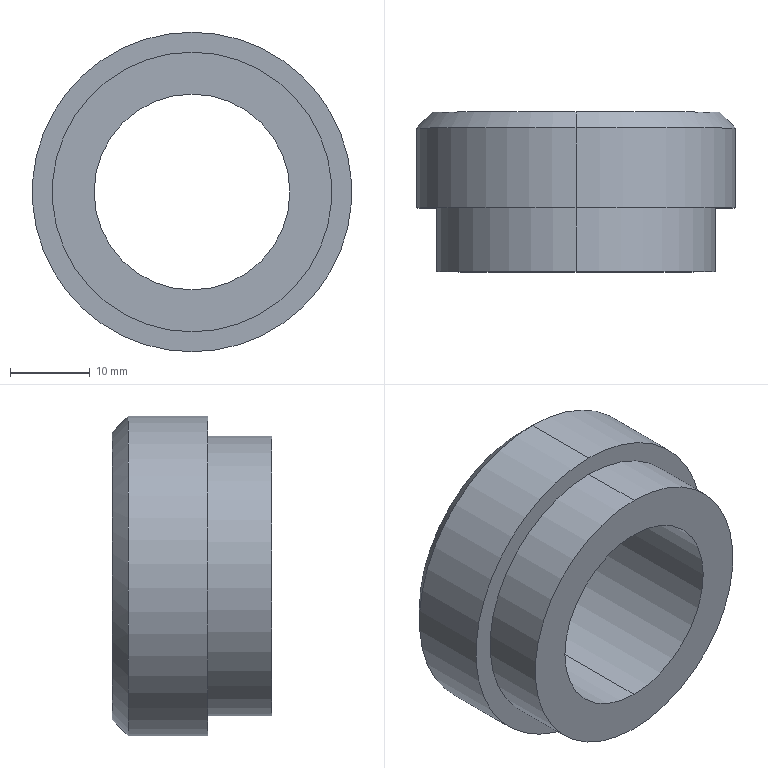Part | SolidWorks | features Chamfer 1, HoleWzd 1, Revolution 1 | 1 solid | 11 faces | box 40 x 20 x 40 mm | volume 13105 mm3 | cylinder 6 | plane 3 | cone 2 | commonest cylinder face diameters 24.5 x2 35 x2 40 x2
STEP:
#1=CARTESIAN_POINT('',(0.,0.,18.));
#2=VERTEX_POINT('',#1);
#3=CARTESIAN_POINT('',(0.,0.,-18.));
#4=VERTEX_POINT('',#3);
#5=CARTESIAN_POINT('',(0.,0.,0.));
#6=DIRECTION('',(0.,1.,0.));
#7=DIRECTION('',(0.,0.,1.));
#8=AXIS2_PLACEMENT_3D('',#5,#6,#7);
#9=CIRCLE('',#8,18.);
#10=EDGE_CURVE('',#2,#4,#9,.T.);
#11=ORIENTED_EDGE('',*,*,#10,.F.);
#12=CARTESIAN_POINT('',(0.,-2.,20.));
#13=VERTEX_POINT('',#12);
#14=CARTESIAN_POINT('',(0.,-2.,20.));
#15=DIRECTION('',(0.,-0.7071,0.7071));
#16=VECTOR('',#15,1000.);
#17=LINE('',#14,#16);
#18=EDGE_CURVE('',#2,#13,#17,.T.);
#19=ORIENTED_EDGE('',*,*,#18,.T.);
#20=CARTESIAN_POINT('',(0.,-2.,-20.));
#21=VERTEX_POINT('',#20);
#22=CARTESIAN_POINT('',(0.,-2.,0.));
#23=DIRECTION('',(0.,-1.,0.));
#24=DIRECTION('',(0.,0.,1.));
#25=AXIS2_PLACEMENT_3D('',#22,#23,#24);
#26=CIRCLE('',#25,20.);
#27=EDGE_CURVE('',#21,#13,#26,.T.);
#28=ORIENTED_EDGE('',*,*,#27,.F.);
#29=CARTESIAN_POINT('',(0.,-2.,-20.));
#30=DIRECTION('',(0.,-0.7071,-0.7071));
#31=VECTOR('',#30,1000.);
#32=LINE('',#29,#31);
#33=EDGE_CURVE('',#4,#21,#32,.T.);
#34=ORIENTED_EDGE('',*,*,#33,.F.);
#35=EDGE_LOOP('',(#11,#19,#28,#34));
#36=FACE_OUTER_BOUND('',#35,.T.);
#37=CARTESIAN_POINT('',(0.,-2.,0.));
#38=DIRECTION('',(0.,-1.,0.));
#39=DIRECTION('',(0.,0.,-1.));
#40=AXIS2_PLACEMENT_3D('',#37,#38,#39);
#41=CONICAL_SURFACE('',#40,20.,0.7854);
#42=ADVANCED_FACE('',(#36),#41,.T.);
#43=CARTESIAN_POINT('',(0.,-20.,12.25));
#44=VERTEX_POINT('',#43);
#45=CARTESIAN_POINT('',(0.,-20.,-12.25));
#46=VERTEX_POINT('',#45);
#47=CARTESIAN_POINT('',(0.,-20.,0.));
#48=DIRECTION('',(0.,-1.,0.));
#49=DIRECTION('',(0.,0.,-1.));
#50=AXIS2_PLACEMENT_3D('',#47,#48,#49);
#51=CIRCLE('',#50,12.25);
#52=EDGE_CURVE('',#44,#46,#51,.T.);
#53=ORIENTED_EDGE('',*,*,#52,.T.);
#54=CARTESIAN_POINT('',(0.,0.,-12.25));
#55=VERTEX_POINT('',#54);
#56=CARTESIAN_POINT('',(0.,0.,-12.25));
#57=DIRECTION('',(0.,1.,0.));
#58=VECTOR('',#57,1000.);
#59=LINE('',#56,#58);
#60=EDGE_CURVE('',#46,#55,#59,.T.);
#61=ORIENTED_EDGE('',*,*,#60,.T.);
#62=CARTESIAN_POINT('',(0.,0.,12.25));
#63=VERTEX_POINT('',#62);
#64=CARTESIAN_POINT('',(0.,0.,0.));
#65=DIRECTION('',(0.,1.,0.));
#66=DIRECTION('',(0.,0.,1.));
#67=AXIS2_PLACEMENT_3D('',#64,#65,#66);
#68=CIRCLE('',#67,12.25);
#69=EDGE_CURVE('',#55,#63,#68,.T.);
#70=ORIENTED_EDGE('',*,*,#69,.T.);
#71=CARTESIAN_POINT('',(0.,0.,12.25));
#72=DIRECTION('',(0.,1.,0.));
#73=VECTOR('',#72,1000.);
#74=LINE('',#71,#73);
#75=EDGE_CURVE('',#44,#63,#74,.T.);
#76=ORIENTED_EDGE('',*,*,#75,.F.);
#77=EDGE_LOOP('',(#53,#61,#70,#76));
#78=FACE_OUTER_BOUND('',#77,.T.);
#79=CARTESIAN_POINT('',(0.,0.,0.));
#80=DIRECTION('',(0.,1.,0.));
#81=DIRECTION('',(0.,0.,1.));
#82=AXIS2_PLACEMENT_3D('',#79,#80,#81);
#83=CYLINDRICAL_SURFACE('',#82,12.25);
#84=ADVANCED_FACE('',(#78),#83,.F.);
#85=CARTESIAN_POINT('',(0.,-12.,-17.5));
#86=VERTEX_POINT('',#85);
#87=CARTESIAN_POINT('',(0.,-12.,17.5));
#88=VERTEX_POINT('',#87);
#89=CARTESIAN_POINT('',(0.,-12.,0.));
#90=DIRECTION('',(0.,-1.,0.));
#91=DIRECTION('',(0.,0.,-1.));
#92=AXIS2_PLACEMENT_3D('',#89,#90,#91);
#93=CIRCLE('',#92,17.5);
#94=EDGE_CURVE('',#86,#88,#93,.T.);
#95=ORIENTED_EDGE('',*,*,#94,.T.);
#96=CARTESIAN_POINT('',(0.,-20.,17.5));
#97=VERTEX_POINT('',#96);
#98=CARTESIAN_POINT('',(0.,-20.,17.5));
#99=DIRECTION('',(0.,-1.,0.));
#100=VECTOR('',#99,1000.);
#101=LINE('',#98,#100);
#102=EDGE_CURVE('',#88,#97,#101,.T.);
#103=ORIENTED_EDGE('',*,*,#102,.T.);
#104=CARTESIAN_POINT('',(0.,-20.,-17.5));
#105=VERTEX_POINT('',#104);
#106=CARTESIAN_POINT('',(0.,-20.,0.));
#107=DIRECTION('',(0.,-1.,0.));
#108=DIRECTION('',(0.,0.,-1.));
#109=AXIS2_PLACEMENT_3D('',#106,#107,#108);
#110=CIRCLE('',#109,17.5);
#111=EDGE_CURVE('',#105,#97,#110,.T.);
#112=ORIENTED_EDGE('',*,*,#111,.F.);
#113=CARTESIAN_POINT('',(0.,-20.,-17.5));
#114=DIRECTION('',(0.,-1.,0.));
#115=VECTOR('',#114,1000.);
#116=LINE('',#113,#115);
#117=EDGE_CURVE('',#86,#105,#116,.T.);
#118=ORIENTED_EDGE('',*,*,#117,.F.);
#119=EDGE_LOOP('',(#95,#103,#112,#118));
#120=FACE_OUTER_BOUND('',#119,.T.);
#121=CARTESIAN_POINT('',(0.,-20.,0.));
#122=DIRECTION('',(0.,-1.,0.));
#123=DIRECTION('',(0.,0.,-1.));
#124=AXIS2_PLACEMENT_3D('',#121,#122,#123);
#125=CYLINDRICAL_SURFACE('',#124,17.5);
#126=ADVANCED_FACE('',(#120),#125,.T.);
#127=ORIENTED_EDGE('',*,*,#27,.T.);
#128=CARTESIAN_POINT('',(0.,-12.,20.));
#129=VERTEX_POINT('',#128);
#130=CARTESIAN_POINT('',(0.,-20.,20.));
#131=DIRECTION('',(0.,-1.,0.));
#132=VECTOR('',#131,1000.);
#133=LINE('',#130,#132);
#134=EDGE_CURVE('',#13,#129,#133,.T.);
#135=ORIENTED_EDGE('',*,*,#134,.T.);
#136=CARTESIAN_POINT('',(0.,-12.,-20.));
#137=VERTEX_POINT('',#136);
#138=CARTESIAN_POINT('',(0.,-12.,0.));
#139=DIRECTION('',(0.,-1.,0.));
#140=DIRECTION('',(0.,0.,-1.));
#141=AXIS2_PLACEMENT_3D('',#138,#139,#140);
#142=CIRCLE('',#141,20.);
#143=EDGE_CURVE('',#137,#129,#142,.T.);
#144=ORIENTED_EDGE('',*,*,#143,.F.);
#145=CARTESIAN_POINT('',(0.,-20.,-20.));
#146=DIRECTION('',(0.,-1.,0.));
#147=VECTOR('',#146,1000.);
#148=LINE('',#145,#147);
#149=EDGE_CURVE('',#21,#137,#148,.T.);
#150=ORIENTED_EDGE('',*,*,#149,.F.);
#151=EDGE_LOOP('',(#127,#135,#144,#150));
#152=FACE_OUTER_BOUND('',#151,.T.);
#153=CARTESIAN_POINT('',(0.,-20.,0.));
#154=DIRECTION('',(0.,-1.,0.));
#155=DIRECTION('',(0.,0.,-1.));
#156=AXIS2_PLACEMENT_3D('',#153,#154,#155);
#157=CYLINDRICAL_SURFACE('',#156,20.);
#158=ADVANCED_FACE('',(#152),#157,.T.);
#159=CARTESIAN_POINT('',(0.,0.,0.));
#160=DIRECTION('',(0.,1.,0.));
#161=DIRECTION('',(0.,0.,1.));
#162=AXIS2_PLACEMENT_3D('',#159,#160,#161);
#163=CIRCLE('',#162,18.);
#164=EDGE_CURVE('',#4,#2,#163,.T.);
#165=ORIENTED_EDGE('',*,*,#164,.T.);
#166=ORIENTED_EDGE('',*,*,#10,.T.);
#167=EDGE_LOOP('',(#165,#166));
#168=FACE_OUTER_BOUND('',#167,.T.);
#169=CARTESIAN_POINT('',(0.,0.,0.));
#170=DIRECTION('',(0.,1.,0.));
#171=DIRECTION('',(0.,0.,1.));
#172=AXIS2_PLACEMENT_3D('',#169,#170,#171);
#173=CIRCLE('',#172,12.25);
#174=EDGE_CURVE('',#63,#55,#173,.T.);
#175=ORIENTED_EDGE('',*,*,#174,.F.);
#176=ORIENTED_EDGE('',*,*,#69,.F.);
#177=EDGE_LOOP('',(#175,#176));
#178=FACE_BOUND('',#177,.T.);
#179=CARTESIAN_POINT('',(0.,0.,0.));
#180=DIRECTION('',(0.,1.,0.));
#181=DIRECTION('',(0.,0.,1.));
#182=AXIS2_PLACEMENT_3D('',#179,#180,#181);
#183=PLANE('',#182);
#184=ADVANCED_FACE('',(#168,#178),#183,.T.);
#185=ORIENTED_EDGE('',*,*,#134,.F.);
#186=CARTESIAN_POINT('',(0.,-2.,0.));
#187=DIRECTION('',(0.,-1.,0.));
#188=DIRECTION('',(0.,0.,1.));
#189=AXIS2_PLACEMENT_3D('',#186,#187,#188);
#190=CIRCLE('',#189,20.);
#191=EDGE_CURVE('',#13,#21,#190,.T.);
#192=ORIENTED_EDGE('',*,*,#191,.T.);
#193=ORIENTED_EDGE('',*,*,#149,.T.);
#194=CARTESIAN_POINT('',(0.,-12.,0.));
#195=DIRECTION('',(0.,-1.,0.));
#196=DIRECTION('',(0.,0.,-1.));
#197=AXIS2_PLACEMENT_3D('',#194,#195,#196);
#198=CIRCLE('',#197,20.);
#199=EDGE_CURVE('',#129,#137,#198,.T.);
#200=ORIENTED_EDGE('',*,*,#199,.F.);
#201=EDGE_LOOP('',(#185,#192,#193,#200));
#202=FACE_OUTER_BOUND('',#201,.T.);
#203=CARTESIAN_POINT('',(0.,-20.,0.));
#204=DIRECTION('',(0.,-1.,0.));
#205=DIRECTION('',(0.,0.,-1.));
#206=AXIS2_PLACEMENT_3D('',#203,#204,#205);
#207=CYLINDRICAL_SURFACE('',#206,20.);
#208=ADVANCED_FACE('',(#202),#207,.T.);
#209=ORIENTED_EDGE('',*,*,#143,.T.);
#210=ORIENTED_EDGE('',*,*,#199,.T.);
#211=EDGE_LOOP('',(#209,#210));
#212=FACE_OUTER_BOUND('',#211,.T.);
#213=ORIENTED_EDGE('',*,*,#94,.F.);
#214=CARTESIAN_POINT('',(0.,-12.,0.));
#215=DIRECTION('',(0.,-1.,0.));
#216=DIRECTION('',(0.,0.,-1.));
#217=AXIS2_PLACEMENT_3D('',#214,#215,#216);
#218=CIRCLE('',#217,17.5);
#219=EDGE_CURVE('',#88,#86,#218,.T.);
#220=ORIENTED_EDGE('',*,*,#219,.F.);
#221=EDGE_LOOP('',(#213,#220));
#222=FACE_BOUND('',#221,.T.);
#223=CARTESIAN_POINT('',(20.,-12.,0.));
#224=DIRECTION('',(0.,-1.,0.));
#225=DIRECTION('',(0.,0.,-1.));
#226=AXIS2_PLACEMENT_3D('',#223,#224,#225);
#227=PLANE('',#226);
#228=ADVANCED_FACE('',(#212,#222),#227,.T.);
#229=ORIENTED_EDGE('',*,*,#102,.F.);
#230=ORIENTED_EDGE('',*,*,#219,.T.);
#231=ORIENTED_EDGE('',*,*,#117,.T.);
#232=CARTESIAN_POINT('',(0.,-20.,0.));
#233=DIRECTION('',(0.,-1.,0.));
#234=DIRECTION('',(0.,0.,-1.));
#235=AXIS2_PLACEMENT_3D('',#232,#233,#234);
#236=CIRCLE('',#235,17.5);
#237=EDGE_CURVE('',#97,#105,#236,.T.);
#238=ORIENTED_EDGE('',*,*,#237,.F.);
#239=EDGE_LOOP('',(#229,#230,#231,#238));
#240=FACE_OUTER_BOUND('',#239,.T.);
#241=CARTESIAN_POINT('',(0.,-20.,0.));
#242=DIRECTION('',(0.,-1.,0.));
#243=DIRECTION('',(0.,0.,-1.));
#244=AXIS2_PLACEMENT_3D('',#241,#242,#243);
#245=CYLINDRICAL_SURFACE('',#244,17.5);
#246=ADVANCED_FACE('',(#240),#245,.T.);
#247=ORIENTED_EDGE('',*,*,#52,.F.);
#248=CARTESIAN_POINT('',(0.,-20.,0.));
#249=DIRECTION('',(0.,-1.,0.));
#250=DIRECTION('',(0.,0.,-1.));
#251=AXIS2_PLACEMENT_3D('',#248,#249,#250);
#252=CIRCLE('',#251,12.25);
#253=EDGE_CURVE('',#46,#44,#252,.T.);
#254=ORIENTED_EDGE('',*,*,#253,.F.);
#255=EDGE_LOOP('',(#247,#254));
#256=FACE_BOUND('',#255,.T.);
#257=ORIENTED_EDGE('',*,*,#111,.T.);
#258=ORIENTED_EDGE('',*,*,#237,.T.);
#259=EDGE_LOOP('',(#257,#258));
#260=FACE_OUTER_BOUND('',#259,.T.);
#261=CARTESIAN_POINT('',(17.5,-20.,0.));
#262=DIRECTION('',(0.,-1.,0.));
#263=DIRECTION('',(0.,0.,-1.));
#264=AXIS2_PLACEMENT_3D('',#261,#262,#263);
#265=PLANE('',#264);
#266=ADVANCED_FACE('',(#256,#260),#265,.T.);
#267=ORIENTED_EDGE('',*,*,#60,.F.);
#268=ORIENTED_EDGE('',*,*,#253,.T.);
#269=ORIENTED_EDGE('',*,*,#75,.T.);
#270=ORIENTED_EDGE('',*,*,#174,.T.);
#271=EDGE_LOOP('',(#267,#268,#269,#270));
#272=FACE_OUTER_BOUND('',#271,.T.);
#273=CARTESIAN_POINT('',(0.,0.,0.));
#274=DIRECTION('',(0.,1.,0.));
#275=DIRECTION('',(0.,0.,1.));
#276=AXIS2_PLACEMENT_3D('',#273,#274,#275);
#277=CYLINDRICAL_SURFACE('',#276,12.25);
#278=ADVANCED_FACE('',(#272),#277,.F.);
#279=ORIENTED_EDGE('',*,*,#18,.F.);
#280=ORIENTED_EDGE('',*,*,#164,.F.);
#281=ORIENTED_EDGE('',*,*,#33,.T.);
#282=ORIENTED_EDGE('',*,*,#191,.F.);
#283=EDGE_LOOP('',(#279,#280,#281,#282));
#284=FACE_OUTER_BOUND('',#283,.T.);
#285=CARTESIAN_POINT('',(0.,-2.,0.));
#286=DIRECTION('',(0.,-1.,0.));
#287=DIRECTION('',(0.,0.,-1.));
#288=AXIS2_PLACEMENT_3D('',#285,#286,#287);
#289=CONICAL_SURFACE('',#288,20.,0.7854);
#290=ADVANCED_FACE('',(#284),#289,.T.);
#291=CLOSED_SHELL('',(#42,#84,#126,#158,#184,#208,#228,#246,#266,#278,#290));
#292=MANIFOLD_SOLID_BREP('',#291);
#293=CARTESIAN_POINT('',(0.,0.,0.));
#294=DIRECTION('',(0.,0.,1.));
#295=DIRECTION('',(1.,0.,0.));
#296=AXIS2_PLACEMENT_3D('',#293,#294,#295);
#297=(LENGTH_UNIT()NAMED_UNIT(*)SI_UNIT(.MILLI.,.METRE.));
#298=UNCERTAINTY_MEASURE_WITH_UNIT(LENGTH_MEASURE(0.00001),#297,'','');
#299=(NAMED_UNIT(*)PLANE_ANGLE_UNIT()SI_UNIT($,.RADIAN.));
#300=(NAMED_UNIT(*)SI_UNIT($,.STERADIAN.)SOLID_ANGLE_UNIT());
#301=(GEOMETRIC_REPRESENTATION_CONTEXT(3)GLOBAL_UNCERTAINTY_ASSIGNED_CONTEXT((#298))GLOBAL_UNIT_ASSIGNED_CONTEXT((#297,#299,#300))REPRESENTATION_CONTEXT('',''));
#302=ADVANCED_BREP_SHAPE_REPRESENTATION('',(#292,#296),#301);